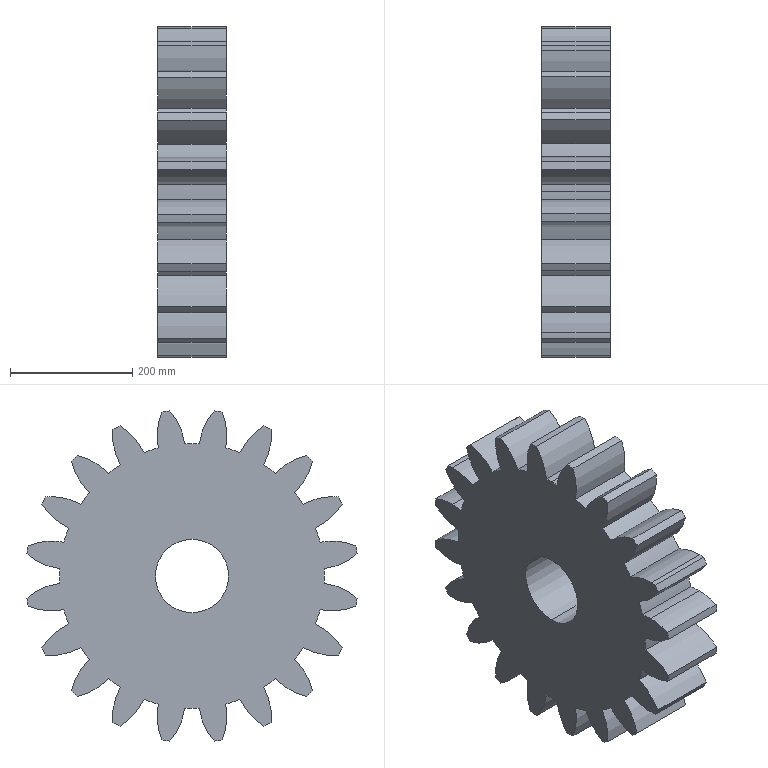Part | SolidWorks | features ICE 2, BaseBody 1, Scale 1 | 1 solid | 89 faces | box 112.2 x 539.706 x 539.706 mm | volume 19588438 mm3 | cylinder 87 | plane 2 | commonest cylinder face diameters 198 x44 433.124 x21 544.5 x20 120 x2